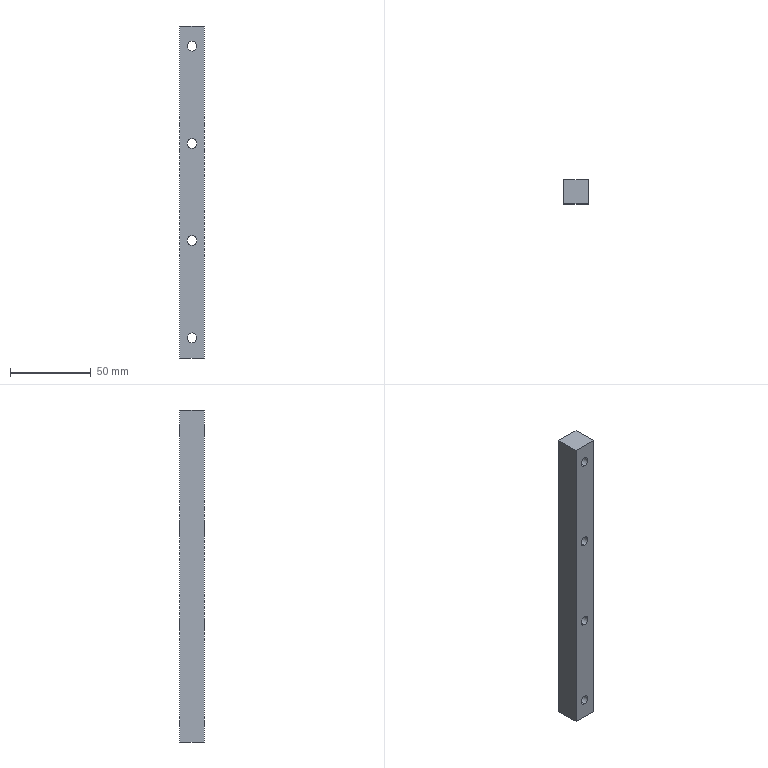Part | 1 solid | 14 faces | box 15 x 15 x 205 mm | volume 44429 mm3 | cylinder 8 | plane 6 | commonest cylinder face diameters 6 x8
STEP:
#1=CARTESIAN_POINT('',(7.5,0.,462.));
#2=VERTEX_POINT('',#1);
#3=CARTESIAN_POINT('',(7.5,0.,468.));
#4=VERTEX_POINT('',#3);
#5=CARTESIAN_POINT('',(7.5,0.,465.));
#6=DIRECTION('',(0.,1.,0.));
#7=DIRECTION('',(0.,0.,1.));
#8=AXIS2_PLACEMENT_3D('',#5,#6,#7);
#9=CIRCLE('',#8,3.);
#10=EDGE_CURVE('',#2,#4,#9,.T.);
#11=ORIENTED_EDGE('',*,*,#10,.F.);
#12=CARTESIAN_POINT('',(7.5,15.,462.));
#13=VERTEX_POINT('',#12);
#14=CARTESIAN_POINT('',(7.5,15.,462.));
#15=DIRECTION('',(0.,1.,0.));
#16=VECTOR('',#15,1000.);
#17=LINE('',#14,#16);
#18=EDGE_CURVE('',#2,#13,#17,.T.);
#19=ORIENTED_EDGE('',*,*,#18,.T.);
#20=CARTESIAN_POINT('',(7.5,15.,468.));
#21=VERTEX_POINT('',#20);
#22=CARTESIAN_POINT('',(7.5,15.,465.));
#23=DIRECTION('',(0.,1.,0.));
#24=DIRECTION('',(0.,0.,1.));
#25=AXIS2_PLACEMENT_3D('',#22,#23,#24);
#26=CIRCLE('',#25,3.);
#27=EDGE_CURVE('',#13,#21,#26,.T.);
#28=ORIENTED_EDGE('',*,*,#27,.T.);
#29=CARTESIAN_POINT('',(7.5,15.,468.));
#30=DIRECTION('',(0.,1.,0.));
#31=VECTOR('',#30,1000.);
#32=LINE('',#29,#31);
#33=EDGE_CURVE('',#4,#21,#32,.T.);
#34=ORIENTED_EDGE('',*,*,#33,.F.);
#35=EDGE_LOOP('',(#11,#19,#28,#34));
#36=FACE_OUTER_BOUND('',#35,.T.);
#37=CARTESIAN_POINT('',(7.5,15.,465.));
#38=DIRECTION('',(0.,1.,0.));
#39=DIRECTION('',(0.,0.,1.));
#40=AXIS2_PLACEMENT_3D('',#37,#38,#39);
#41=CYLINDRICAL_SURFACE('',#40,3.);
#42=ADVANCED_FACE('',(#36),#41,.F.);
#43=CARTESIAN_POINT('',(7.5,0.,402.));
#44=VERTEX_POINT('',#43);
#45=CARTESIAN_POINT('',(7.5,0.,408.));
#46=VERTEX_POINT('',#45);
#47=CARTESIAN_POINT('',(7.5,0.,405.));
#48=DIRECTION('',(0.,1.,0.));
#49=DIRECTION('',(0.,0.,1.));
#50=AXIS2_PLACEMENT_3D('',#47,#48,#49);
#51=CIRCLE('',#50,3.);
#52=EDGE_CURVE('',#44,#46,#51,.T.);
#53=ORIENTED_EDGE('',*,*,#52,.F.);
#54=CARTESIAN_POINT('',(7.5,15.,402.));
#55=VERTEX_POINT('',#54);
#56=CARTESIAN_POINT('',(7.5,15.,402.));
#57=DIRECTION('',(0.,1.,0.));
#58=VECTOR('',#57,1000.);
#59=LINE('',#56,#58);
#60=EDGE_CURVE('',#44,#55,#59,.T.);
#61=ORIENTED_EDGE('',*,*,#60,.T.);
#62=CARTESIAN_POINT('',(7.5,15.,408.));
#63=VERTEX_POINT('',#62);
#64=CARTESIAN_POINT('',(7.5,15.,405.));
#65=DIRECTION('',(0.,1.,0.));
#66=DIRECTION('',(0.,0.,1.));
#67=AXIS2_PLACEMENT_3D('',#64,#65,#66);
#68=CIRCLE('',#67,3.);
#69=EDGE_CURVE('',#55,#63,#68,.T.);
#70=ORIENTED_EDGE('',*,*,#69,.T.);
#71=CARTESIAN_POINT('',(7.5,15.,408.));
#72=DIRECTION('',(0.,1.,0.));
#73=VECTOR('',#72,1000.);
#74=LINE('',#71,#73);
#75=EDGE_CURVE('',#46,#63,#74,.T.);
#76=ORIENTED_EDGE('',*,*,#75,.F.);
#77=EDGE_LOOP('',(#53,#61,#70,#76));
#78=FACE_OUTER_BOUND('',#77,.T.);
#79=CARTESIAN_POINT('',(7.5,15.,405.));
#80=DIRECTION('',(0.,1.,0.));
#81=DIRECTION('',(0.,0.,1.));
#82=AXIS2_PLACEMENT_3D('',#79,#80,#81);
#83=CYLINDRICAL_SURFACE('',#82,3.);
#84=ADVANCED_FACE('',(#78),#83,.F.);
#85=CARTESIAN_POINT('',(7.5,0.,342.));
#86=VERTEX_POINT('',#85);
#87=CARTESIAN_POINT('',(7.5,0.,348.));
#88=VERTEX_POINT('',#87);
#89=CARTESIAN_POINT('',(7.5,0.,345.));
#90=DIRECTION('',(0.,1.,0.));
#91=DIRECTION('',(0.,0.,1.));
#92=AXIS2_PLACEMENT_3D('',#89,#90,#91);
#93=CIRCLE('',#92,3.);
#94=EDGE_CURVE('',#86,#88,#93,.T.);
#95=ORIENTED_EDGE('',*,*,#94,.F.);
#96=CARTESIAN_POINT('',(7.5,15.,342.));
#97=VERTEX_POINT('',#96);
#98=CARTESIAN_POINT('',(7.5,15.,342.));
#99=DIRECTION('',(0.,1.,0.));
#100=VECTOR('',#99,1000.);
#101=LINE('',#98,#100);
#102=EDGE_CURVE('',#86,#97,#101,.T.);
#103=ORIENTED_EDGE('',*,*,#102,.T.);
#104=CARTESIAN_POINT('',(7.5,15.,348.));
#105=VERTEX_POINT('',#104);
#106=CARTESIAN_POINT('',(7.5,15.,345.));
#107=DIRECTION('',(0.,1.,0.));
#108=DIRECTION('',(0.,0.,1.));
#109=AXIS2_PLACEMENT_3D('',#106,#107,#108);
#110=CIRCLE('',#109,3.);
#111=EDGE_CURVE('',#97,#105,#110,.T.);
#112=ORIENTED_EDGE('',*,*,#111,.T.);
#113=CARTESIAN_POINT('',(7.5,15.,348.));
#114=DIRECTION('',(0.,1.,0.));
#115=VECTOR('',#114,1000.);
#116=LINE('',#113,#115);
#117=EDGE_CURVE('',#88,#105,#116,.T.);
#118=ORIENTED_EDGE('',*,*,#117,.F.);
#119=EDGE_LOOP('',(#95,#103,#112,#118));
#120=FACE_OUTER_BOUND('',#119,.T.);
#121=CARTESIAN_POINT('',(7.5,15.,345.));
#122=DIRECTION('',(0.,1.,0.));
#123=DIRECTION('',(0.,0.,1.));
#124=AXIS2_PLACEMENT_3D('',#121,#122,#123);
#125=CYLINDRICAL_SURFACE('',#124,3.);
#126=ADVANCED_FACE('',(#120),#125,.F.);
#127=CARTESIAN_POINT('',(7.5,0.,282.));
#128=VERTEX_POINT('',#127);
#129=CARTESIAN_POINT('',(7.5,0.,288.));
#130=VERTEX_POINT('',#129);
#131=CARTESIAN_POINT('',(7.5,0.,285.));
#132=DIRECTION('',(0.,1.,0.));
#133=DIRECTION('',(0.,0.,1.));
#134=AXIS2_PLACEMENT_3D('',#131,#132,#133);
#135=CIRCLE('',#134,3.);
#136=EDGE_CURVE('',#128,#130,#135,.T.);
#137=ORIENTED_EDGE('',*,*,#136,.F.);
#138=CARTESIAN_POINT('',(7.5,15.,282.));
#139=VERTEX_POINT('',#138);
#140=CARTESIAN_POINT('',(7.5,15.,282.));
#141=DIRECTION('',(0.,1.,0.));
#142=VECTOR('',#141,1000.);
#143=LINE('',#140,#142);
#144=EDGE_CURVE('',#128,#139,#143,.T.);
#145=ORIENTED_EDGE('',*,*,#144,.T.);
#146=CARTESIAN_POINT('',(7.5,15.,288.));
#147=VERTEX_POINT('',#146);
#148=CARTESIAN_POINT('',(7.5,15.,285.));
#149=DIRECTION('',(0.,1.,0.));
#150=DIRECTION('',(0.,0.,1.));
#151=AXIS2_PLACEMENT_3D('',#148,#149,#150);
#152=CIRCLE('',#151,3.);
#153=EDGE_CURVE('',#139,#147,#152,.T.);
#154=ORIENTED_EDGE('',*,*,#153,.T.);
#155=CARTESIAN_POINT('',(7.5,15.,288.));
#156=DIRECTION('',(0.,1.,0.));
#157=VECTOR('',#156,1000.);
#158=LINE('',#155,#157);
#159=EDGE_CURVE('',#130,#147,#158,.T.);
#160=ORIENTED_EDGE('',*,*,#159,.F.);
#161=EDGE_LOOP('',(#137,#145,#154,#160));
#162=FACE_OUTER_BOUND('',#161,.T.);
#163=CARTESIAN_POINT('',(7.5,15.,285.));
#164=DIRECTION('',(0.,1.,0.));
#165=DIRECTION('',(0.,0.,1.));
#166=AXIS2_PLACEMENT_3D('',#163,#164,#165);
#167=CYLINDRICAL_SURFACE('',#166,3.);
#168=ADVANCED_FACE('',(#162),#167,.F.);
#169=CARTESIAN_POINT('',(0.,15.,477.5));
#170=VERTEX_POINT('',#169);
#171=CARTESIAN_POINT('',(0.,15.,272.5));
#172=VERTEX_POINT('',#171);
#173=CARTESIAN_POINT('',(0.,15.,720.));
#174=DIRECTION('',(0.,0.,-1.));
#175=VECTOR('',#174,1000.);
#176=LINE('',#173,#175);
#177=EDGE_CURVE('',#170,#172,#176,.T.);
#178=ORIENTED_EDGE('',*,*,#177,.T.);
#179=CARTESIAN_POINT('',(0.,0.,272.5));
#180=VERTEX_POINT('',#179);
#181=CARTESIAN_POINT('',(0.,0.,272.5));
#182=DIRECTION('',(0.,1.,0.));
#183=VECTOR('',#182,1000.);
#184=LINE('',#181,#183);
#185=EDGE_CURVE('',#180,#172,#184,.T.);
#186=ORIENTED_EDGE('',*,*,#185,.F.);
#187=CARTESIAN_POINT('',(0.,0.,477.5));
#188=VERTEX_POINT('',#187);
#189=CARTESIAN_POINT('',(0.,0.,720.));
#190=DIRECTION('',(0.,0.,-1.));
#191=VECTOR('',#190,1000.);
#192=LINE('',#189,#191);
#193=EDGE_CURVE('',#188,#180,#192,.T.);
#194=ORIENTED_EDGE('',*,*,#193,.F.);
#195=CARTESIAN_POINT('',(0.,0.,477.5));
#196=DIRECTION('',(0.,1.,0.));
#197=VECTOR('',#196,1000.);
#198=LINE('',#195,#197);
#199=EDGE_CURVE('',#188,#170,#198,.T.);
#200=ORIENTED_EDGE('',*,*,#199,.T.);
#201=EDGE_LOOP('',(#178,#186,#194,#200));
#202=FACE_OUTER_BOUND('',#201,.T.);
#203=CARTESIAN_POINT('',(0.,0.,720.));
#204=DIRECTION('',(1.,0.,0.));
#205=DIRECTION('',(0.,0.,-1.));
#206=AXIS2_PLACEMENT_3D('',#203,#204,#205);
#207=PLANE('',#206);
#208=ADVANCED_FACE('',(#202),#207,.F.);
#209=CARTESIAN_POINT('',(7.5,0.,465.));
#210=DIRECTION('',(0.,1.,0.));
#211=DIRECTION('',(0.,0.,1.));
#212=AXIS2_PLACEMENT_3D('',#209,#210,#211);
#213=CIRCLE('',#212,3.);
#214=EDGE_CURVE('',#4,#2,#213,.T.);
#215=ORIENTED_EDGE('',*,*,#214,.T.);
#216=ORIENTED_EDGE('',*,*,#10,.T.);
#217=EDGE_LOOP('',(#215,#216));
#218=FACE_BOUND('',#217,.T.);
#219=CARTESIAN_POINT('',(7.5,0.,405.));
#220=DIRECTION('',(0.,1.,0.));
#221=DIRECTION('',(0.,0.,1.));
#222=AXIS2_PLACEMENT_3D('',#219,#220,#221);
#223=CIRCLE('',#222,3.);
#224=EDGE_CURVE('',#46,#44,#223,.T.);
#225=ORIENTED_EDGE('',*,*,#224,.T.);
#226=ORIENTED_EDGE('',*,*,#52,.T.);
#227=EDGE_LOOP('',(#225,#226));
#228=FACE_BOUND('',#227,.T.);
#229=CARTESIAN_POINT('',(7.5,0.,345.));
#230=DIRECTION('',(0.,1.,0.));
#231=DIRECTION('',(0.,0.,1.));
#232=AXIS2_PLACEMENT_3D('',#229,#230,#231);
#233=CIRCLE('',#232,3.);
#234=EDGE_CURVE('',#88,#86,#233,.T.);
#235=ORIENTED_EDGE('',*,*,#234,.T.);
#236=ORIENTED_EDGE('',*,*,#94,.T.);
#237=EDGE_LOOP('',(#235,#236));
#238=FACE_BOUND('',#237,.T.);
#239=CARTESIAN_POINT('',(7.5,0.,285.));
#240=DIRECTION('',(0.,1.,0.));
#241=DIRECTION('',(0.,0.,1.));
#242=AXIS2_PLACEMENT_3D('',#239,#240,#241);
#243=CIRCLE('',#242,3.);
#244=EDGE_CURVE('',#130,#128,#243,.T.);
#245=ORIENTED_EDGE('',*,*,#244,.T.);
#246=ORIENTED_EDGE('',*,*,#136,.T.);
#247=EDGE_LOOP('',(#245,#246));
#248=FACE_BOUND('',#247,.T.);
#249=ORIENTED_EDGE('',*,*,#193,.T.);
#250=CARTESIAN_POINT('',(15.,0.,272.5));
#251=VERTEX_POINT('',#250);
#252=CARTESIAN_POINT('',(0.,0.,272.5));
#253=DIRECTION('',(1.,0.,0.));
#254=VECTOR('',#253,1000.);
#255=LINE('',#252,#254);
#256=EDGE_CURVE('',#180,#251,#255,.T.);
#257=ORIENTED_EDGE('',*,*,#256,.T.);
#258=CARTESIAN_POINT('',(15.,0.,477.5));
#259=VERTEX_POINT('',#258);
#260=CARTESIAN_POINT('',(15.,0.,720.));
#261=DIRECTION('',(0.,0.,-1.));
#262=VECTOR('',#261,1000.);
#263=LINE('',#260,#262);
#264=EDGE_CURVE('',#259,#251,#263,.T.);
#265=ORIENTED_EDGE('',*,*,#264,.F.);
#266=CARTESIAN_POINT('',(0.,0.,477.5));
#267=DIRECTION('',(-1.,0.,0.));
#268=VECTOR('',#267,1000.);
#269=LINE('',#266,#268);
#270=EDGE_CURVE('',#259,#188,#269,.T.);
#271=ORIENTED_EDGE('',*,*,#270,.T.);
#272=EDGE_LOOP('',(#249,#257,#265,#271));
#273=FACE_OUTER_BOUND('',#272,.T.);
#274=CARTESIAN_POINT('',(0.,0.,720.));
#275=DIRECTION('',(0.,1.,0.));
#276=DIRECTION('',(0.,0.,1.));
#277=AXIS2_PLACEMENT_3D('',#274,#275,#276);
#278=PLANE('',#277);
#279=ADVANCED_FACE('',(#218,#228,#238,#248,#273),#278,.F.);
#280=ORIENTED_EDGE('',*,*,#264,.T.);
#281=CARTESIAN_POINT('',(15.,15.,272.5));
#282=VERTEX_POINT('',#281);
#283=CARTESIAN_POINT('',(15.,0.,272.5));
#284=DIRECTION('',(0.,1.,0.));
#285=VECTOR('',#284,1000.);
#286=LINE('',#283,#285);
#287=EDGE_CURVE('',#251,#282,#286,.T.);
#288=ORIENTED_EDGE('',*,*,#287,.T.);
#289=CARTESIAN_POINT('',(15.,15.,477.5));
#290=VERTEX_POINT('',#289);
#291=CARTESIAN_POINT('',(15.,15.,720.));
#292=DIRECTION('',(0.,0.,-1.));
#293=VECTOR('',#292,1000.);
#294=LINE('',#291,#293);
#295=EDGE_CURVE('',#290,#282,#294,.T.);
#296=ORIENTED_EDGE('',*,*,#295,.F.);
#297=CARTESIAN_POINT('',(15.,0.,477.5));
#298=DIRECTION('',(0.,1.,0.));
#299=VECTOR('',#298,1000.);
#300=LINE('',#297,#299);
#301=EDGE_CURVE('',#259,#290,#300,.T.);
#302=ORIENTED_EDGE('',*,*,#301,.F.);
#303=EDGE_LOOP('',(#280,#288,#296,#302));
#304=FACE_OUTER_BOUND('',#303,.T.);
#305=CARTESIAN_POINT('',(15.,0.,720.));
#306=DIRECTION('',(-1.,0.,0.));
#307=DIRECTION('',(0.,0.,1.));
#308=AXIS2_PLACEMENT_3D('',#305,#306,#307);
#309=PLANE('',#308);
#310=ADVANCED_FACE('',(#304),#309,.F.);
#311=CARTESIAN_POINT('',(7.5,15.,465.));
#312=DIRECTION('',(0.,1.,0.));
#313=DIRECTION('',(0.,0.,1.));
#314=AXIS2_PLACEMENT_3D('',#311,#312,#313);
#315=CIRCLE('',#314,3.);
#316=EDGE_CURVE('',#21,#13,#315,.T.);
#317=ORIENTED_EDGE('',*,*,#316,.F.);
#318=ORIENTED_EDGE('',*,*,#27,.F.);
#319=EDGE_LOOP('',(#317,#318));
#320=FACE_BOUND('',#319,.T.);
#321=CARTESIAN_POINT('',(7.5,15.,405.));
#322=DIRECTION('',(0.,1.,0.));
#323=DIRECTION('',(0.,0.,1.));
#324=AXIS2_PLACEMENT_3D('',#321,#322,#323);
#325=CIRCLE('',#324,3.);
#326=EDGE_CURVE('',#63,#55,#325,.T.);
#327=ORIENTED_EDGE('',*,*,#326,.F.);
#328=ORIENTED_EDGE('',*,*,#69,.F.);
#329=EDGE_LOOP('',(#327,#328));
#330=FACE_BOUND('',#329,.T.);
#331=CARTESIAN_POINT('',(7.5,15.,345.));
#332=DIRECTION('',(0.,1.,0.));
#333=DIRECTION('',(0.,0.,1.));
#334=AXIS2_PLACEMENT_3D('',#331,#332,#333);
#335=CIRCLE('',#334,3.);
#336=EDGE_CURVE('',#105,#97,#335,.T.);
#337=ORIENTED_EDGE('',*,*,#336,.F.);
#338=ORIENTED_EDGE('',*,*,#111,.F.);
#339=EDGE_LOOP('',(#337,#338));
#340=FACE_BOUND('',#339,.T.);
#341=CARTESIAN_POINT('',(7.5,15.,285.));
#342=DIRECTION('',(0.,1.,0.));
#343=DIRECTION('',(0.,0.,1.));
#344=AXIS2_PLACEMENT_3D('',#341,#342,#343);
#345=CIRCLE('',#344,3.);
#346=EDGE_CURVE('',#147,#139,#345,.T.);
#347=ORIENTED_EDGE('',*,*,#346,.F.);
#348=ORIENTED_EDGE('',*,*,#153,.F.);
#349=EDGE_LOOP('',(#347,#348));
#350=FACE_BOUND('',#349,.T.);
#351=ORIENTED_EDGE('',*,*,#295,.T.);
#352=CARTESIAN_POINT('',(0.,15.,272.5));
#353=DIRECTION('',(1.,0.,0.));
#354=VECTOR('',#353,1000.);
#355=LINE('',#352,#354);
#356=EDGE_CURVE('',#172,#282,#355,.T.);
#357=ORIENTED_EDGE('',*,*,#356,.F.);
#358=ORIENTED_EDGE('',*,*,#177,.F.);
#359=CARTESIAN_POINT('',(0.,15.,477.5));
#360=DIRECTION('',(-1.,0.,0.));
#361=VECTOR('',#360,1000.);
#362=LINE('',#359,#361);
#363=EDGE_CURVE('',#290,#170,#362,.T.);
#364=ORIENTED_EDGE('',*,*,#363,.F.);
#365=EDGE_LOOP('',(#351,#357,#358,#364));
#366=FACE_OUTER_BOUND('',#365,.T.);
#367=CARTESIAN_POINT('',(0.,15.,720.));
#368=DIRECTION('',(0.,-1.,0.));
#369=DIRECTION('',(0.,0.,-1.));
#370=AXIS2_PLACEMENT_3D('',#367,#368,#369);
#371=PLANE('',#370);
#372=ADVANCED_FACE('',(#320,#330,#340,#350,#366),#371,.F.);
#373=ORIENTED_EDGE('',*,*,#363,.T.);
#374=ORIENTED_EDGE('',*,*,#199,.F.);
#375=ORIENTED_EDGE('',*,*,#270,.F.);
#376=ORIENTED_EDGE('',*,*,#301,.T.);
#377=EDGE_LOOP('',(#373,#374,#375,#376));
#378=FACE_OUTER_BOUND('',#377,.T.);
#379=CARTESIAN_POINT('',(0.,0.,477.5));
#380=DIRECTION('',(0.,0.,-1.));
#381=DIRECTION('',(-1.,0.,0.));
#382=AXIS2_PLACEMENT_3D('',#379,#380,#381);
#383=PLANE('',#382);
#384=ADVANCED_FACE('',(#378),#383,.F.);
#385=ORIENTED_EDGE('',*,*,#356,.T.);
#386=ORIENTED_EDGE('',*,*,#287,.F.);
#387=ORIENTED_EDGE('',*,*,#256,.F.);
#388=ORIENTED_EDGE('',*,*,#185,.T.);
#389=EDGE_LOOP('',(#385,#386,#387,#388));
#390=FACE_OUTER_BOUND('',#389,.T.);
#391=CARTESIAN_POINT('',(0.,0.,272.5));
#392=DIRECTION('',(0.,0.,1.));
#393=DIRECTION('',(1.,0.,0.));
#394=AXIS2_PLACEMENT_3D('',#391,#392,#393);
#395=PLANE('',#394);
#396=ADVANCED_FACE('',(#390),#395,.F.);
#397=ORIENTED_EDGE('',*,*,#144,.F.);
#398=ORIENTED_EDGE('',*,*,#244,.F.);
#399=ORIENTED_EDGE('',*,*,#159,.T.);
#400=ORIENTED_EDGE('',*,*,#346,.T.);
#401=EDGE_LOOP('',(#397,#398,#399,#400));
#402=FACE_OUTER_BOUND('',#401,.T.);
#403=CARTESIAN_POINT('',(7.5,15.,285.));
#404=DIRECTION('',(0.,1.,0.));
#405=DIRECTION('',(0.,0.,1.));
#406=AXIS2_PLACEMENT_3D('',#403,#404,#405);
#407=CYLINDRICAL_SURFACE('',#406,3.);
#408=ADVANCED_FACE('',(#402),#407,.F.);
#409=ORIENTED_EDGE('',*,*,#102,.F.);
#410=ORIENTED_EDGE('',*,*,#234,.F.);
#411=ORIENTED_EDGE('',*,*,#117,.T.);
#412=ORIENTED_EDGE('',*,*,#336,.T.);
#413=EDGE_LOOP('',(#409,#410,#411,#412));
#414=FACE_OUTER_BOUND('',#413,.T.);
#415=CARTESIAN_POINT('',(7.5,15.,345.));
#416=DIRECTION('',(0.,1.,0.));
#417=DIRECTION('',(0.,0.,1.));
#418=AXIS2_PLACEMENT_3D('',#415,#416,#417);
#419=CYLINDRICAL_SURFACE('',#418,3.);
#420=ADVANCED_FACE('',(#414),#419,.F.);
#421=ORIENTED_EDGE('',*,*,#60,.F.);
#422=ORIENTED_EDGE('',*,*,#224,.F.);
#423=ORIENTED_EDGE('',*,*,#75,.T.);
#424=ORIENTED_EDGE('',*,*,#326,.T.);
#425=EDGE_LOOP('',(#421,#422,#423,#424));
#426=FACE_OUTER_BOUND('',#425,.T.);
#427=CARTESIAN_POINT('',(7.5,15.,405.));
#428=DIRECTION('',(0.,1.,0.));
#429=DIRECTION('',(0.,0.,1.));
#430=AXIS2_PLACEMENT_3D('',#427,#428,#429);
#431=CYLINDRICAL_SURFACE('',#430,3.);
#432=ADVANCED_FACE('',(#426),#431,.F.);
#433=ORIENTED_EDGE('',*,*,#18,.F.);
#434=ORIENTED_EDGE('',*,*,#214,.F.);
#435=ORIENTED_EDGE('',*,*,#33,.T.);
#436=ORIENTED_EDGE('',*,*,#316,.T.);
#437=EDGE_LOOP('',(#433,#434,#435,#436));
#438=FACE_OUTER_BOUND('',#437,.T.);
#439=CARTESIAN_POINT('',(7.5,15.,465.));
#440=DIRECTION('',(0.,1.,0.));
#441=DIRECTION('',(0.,0.,1.));
#442=AXIS2_PLACEMENT_3D('',#439,#440,#441);
#443=CYLINDRICAL_SURFACE('',#442,3.);
#444=ADVANCED_FACE('',(#438),#443,.F.);
#445=CLOSED_SHELL('',(#42,#84,#126,#168,#208,#279,#310,#372,#384,#396,#408,#420,#432,#444));
#446=MANIFOLD_SOLID_BREP('',#445);
#447=CARTESIAN_POINT('',(0.,0.,0.));
#448=DIRECTION('',(0.,0.,1.));
#449=DIRECTION('',(1.,0.,0.));
#450=AXIS2_PLACEMENT_3D('',#447,#448,#449);
#451=(LENGTH_UNIT()NAMED_UNIT(*)SI_UNIT(.MILLI.,.METRE.));
#452=UNCERTAINTY_MEASURE_WITH_UNIT(LENGTH_MEASURE(0.00001),#451,'','');
#453=(NAMED_UNIT(*)PLANE_ANGLE_UNIT()SI_UNIT($,.RADIAN.));
#454=(NAMED_UNIT(*)SI_UNIT($,.STERADIAN.)SOLID_ANGLE_UNIT());
#455=(GEOMETRIC_REPRESENTATION_CONTEXT(3)GLOBAL_UNCERTAINTY_ASSIGNED_CONTEXT((#452))GLOBAL_UNIT_ASSIGNED_CONTEXT((#451,#453,#454))REPRESENTATION_CONTEXT('',''));
#456=ADVANCED_BREP_SHAPE_REPRESENTATION('',(#446,#450),#455);